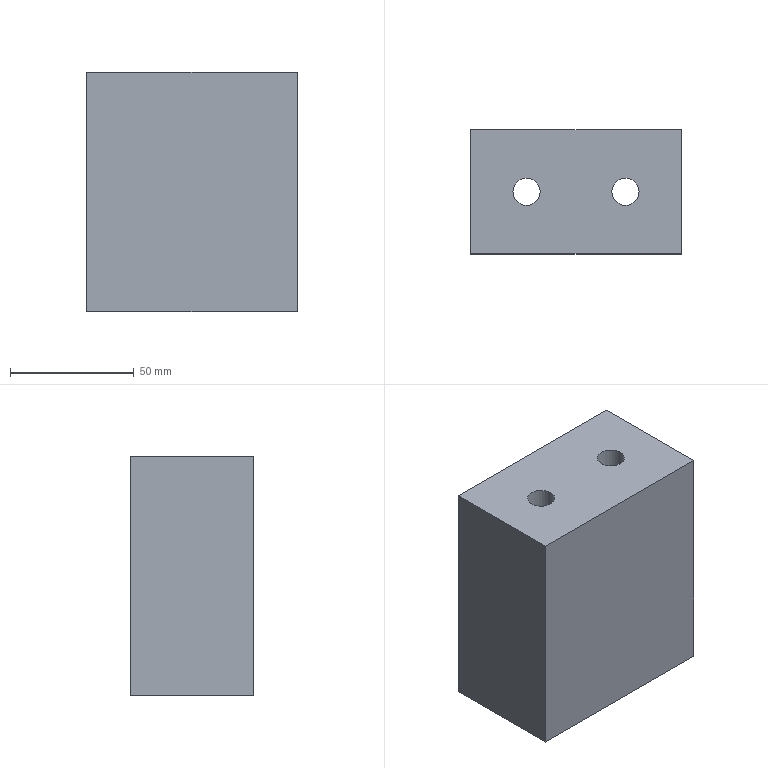Part | STEP file | PN_0040_id1406_x_t | 1 solid | 12 faces | box 85 x 50 x 97 mm | volume 372174 mm3 | plane 8 | cylinder 4 | commonest cylinder face diameters 11 x2 17 x2
STEP:
#1=CARTESIAN_POINT('',(-370.,-242.5,105.));
#2=VERTEX_POINT('',#1);
#3=CARTESIAN_POINT('',(-285.,-242.5,105.));
#4=VERTEX_POINT('',#3);
#5=CARTESIAN_POINT('',(-327.5,-242.5,105.));
#6=DIRECTION('',(1.,0.,0.));
#7=VECTOR('',#6,1.);
#8=LINE('',#5,#7);
#9=EDGE_CURVE('',#2,#4,#8,.T.);
#10=ORIENTED_EDGE('',*,*,#9,.T.);
#11=CARTESIAN_POINT('',(-285.,-242.5,8.));
#12=VERTEX_POINT('',#11);
#13=CARTESIAN_POINT('',(-285.,-242.5,6.));
#14=DIRECTION('',(0.,0.,-1.));
#15=VECTOR('',#14,1.);
#16=LINE('',#13,#15);
#17=EDGE_CURVE('',#4,#12,#16,.T.);
#18=ORIENTED_EDGE('',*,*,#17,.T.);
#19=CARTESIAN_POINT('',(-370.,-242.5,8.));
#20=VERTEX_POINT('',#19);
#21=CARTESIAN_POINT('',(-327.5,-242.5,8.));
#22=DIRECTION('',(-1.,0.,0.));
#23=VECTOR('',#22,1.);
#24=LINE('',#21,#23);
#25=EDGE_CURVE('',#12,#20,#24,.T.);
#26=ORIENTED_EDGE('',*,*,#25,.T.);
#27=CARTESIAN_POINT('',(-370.,-242.5,6.));
#28=DIRECTION('',(0.,0.,-1.));
#29=VECTOR('',#28,1.);
#30=LINE('',#27,#29);
#31=EDGE_CURVE('',#2,#20,#30,.T.);
#32=ORIENTED_EDGE('',*,*,#31,.F.);
#33=EDGE_LOOP('',(#10,#18,#26,#32));
#34=FACE_OUTER_BOUND('',#33,.T.);
#35=CARTESIAN_POINT('',(-327.5,-242.5,6.));
#36=DIRECTION('',(0.,1.,0.));
#37=DIRECTION('',(0.,0.,1.));
#38=AXIS2_PLACEMENT_3D('',#35,#36,#37);
#39=PLANE('',#38);
#40=ADVANCED_FACE('',(#34),#39,.T.);
#41=CARTESIAN_POINT('',(-370.,-292.5,105.));
#42=VERTEX_POINT('',#41);
#43=CARTESIAN_POINT('',(-370.,-267.5,105.));
#44=DIRECTION('',(0.,1.,0.));
#45=VECTOR('',#44,1.);
#46=LINE('',#43,#45);
#47=EDGE_CURVE('',#42,#2,#46,.T.);
#48=ORIENTED_EDGE('',*,*,#47,.T.);
#49=ORIENTED_EDGE('',*,*,#31,.T.);
#50=CARTESIAN_POINT('',(-370.,-292.5,8.));
#51=VERTEX_POINT('',#50);
#52=CARTESIAN_POINT('',(-370.,-267.5,8.));
#53=DIRECTION('',(0.,-1.,0.));
#54=VECTOR('',#53,1.);
#55=LINE('',#52,#54);
#56=EDGE_CURVE('',#20,#51,#55,.T.);
#57=ORIENTED_EDGE('',*,*,#56,.T.);
#58=CARTESIAN_POINT('',(-370.,-292.5,6.));
#59=DIRECTION('',(0.,0.,-1.));
#60=VECTOR('',#59,1.);
#61=LINE('',#58,#60);
#62=EDGE_CURVE('',#42,#51,#61,.T.);
#63=ORIENTED_EDGE('',*,*,#62,.F.);
#64=EDGE_LOOP('',(#48,#49,#57,#63));
#65=FACE_OUTER_BOUND('',#64,.T.);
#66=CARTESIAN_POINT('',(-370.,-267.5,6.));
#67=DIRECTION('',(-1.,0.,0.));
#68=DIRECTION('',(0.,0.,1.));
#69=AXIS2_PLACEMENT_3D('',#66,#67,#68);
#70=PLANE('',#69);
#71=ADVANCED_FACE('',(#65),#70,.T.);
#72=CARTESIAN_POINT('',(-285.,-292.5,8.));
#73=VERTEX_POINT('',#72);
#74=CARTESIAN_POINT('',(-327.5,-292.5,8.));
#75=DIRECTION('',(1.,0.,0.));
#76=VECTOR('',#75,1.);
#77=LINE('',#74,#76);
#78=EDGE_CURVE('',#51,#73,#77,.T.);
#79=ORIENTED_EDGE('',*,*,#78,.T.);
#80=CARTESIAN_POINT('',(-285.,-292.5,105.));
#81=VERTEX_POINT('',#80);
#82=CARTESIAN_POINT('',(-285.,-292.5,6.));
#83=DIRECTION('',(0.,0.,-1.));
#84=VECTOR('',#83,1.);
#85=LINE('',#82,#84);
#86=EDGE_CURVE('',#81,#73,#85,.T.);
#87=ORIENTED_EDGE('',*,*,#86,.F.);
#88=CARTESIAN_POINT('',(-327.5,-292.5,105.));
#89=DIRECTION('',(-1.,0.,0.));
#90=VECTOR('',#89,1.);
#91=LINE('',#88,#90);
#92=EDGE_CURVE('',#81,#42,#91,.T.);
#93=ORIENTED_EDGE('',*,*,#92,.T.);
#94=ORIENTED_EDGE('',*,*,#62,.T.);
#95=EDGE_LOOP('',(#79,#87,#93,#94));
#96=FACE_OUTER_BOUND('',#95,.T.);
#97=CARTESIAN_POINT('',(-327.5,-292.5,6.));
#98=DIRECTION('',(0.,-1.,0.));
#99=DIRECTION('',(0.,0.,-1.));
#100=AXIS2_PLACEMENT_3D('',#97,#98,#99);
#101=PLANE('',#100);
#102=ADVANCED_FACE('',(#96),#101,.T.);
#103=CARTESIAN_POINT('',(-285.,-267.5,8.));
#104=DIRECTION('',(0.,1.,0.));
#105=VECTOR('',#104,1.);
#106=LINE('',#103,#105);
#107=EDGE_CURVE('',#73,#12,#106,.T.);
#108=ORIENTED_EDGE('',*,*,#107,.T.);
#109=ORIENTED_EDGE('',*,*,#17,.F.);
#110=CARTESIAN_POINT('',(-285.,-267.5,105.));
#111=DIRECTION('',(0.,-1.,0.));
#112=VECTOR('',#111,1.);
#113=LINE('',#110,#112);
#114=EDGE_CURVE('',#4,#81,#113,.T.);
#115=ORIENTED_EDGE('',*,*,#114,.T.);
#116=ORIENTED_EDGE('',*,*,#86,.T.);
#117=EDGE_LOOP('',(#108,#109,#115,#116));
#118=FACE_OUTER_BOUND('',#117,.T.);
#119=CARTESIAN_POINT('',(-285.,-267.5,6.));
#120=DIRECTION('',(1.,0.,0.));
#121=DIRECTION('',(0.,0.,-1.));
#122=AXIS2_PLACEMENT_3D('',#119,#120,#121);
#123=PLANE('',#122);
#124=ADVANCED_FACE('',(#118),#123,.T.);
#125=CARTESIAN_POINT('',(-356.,-267.5,8.));
#126=VERTEX_POINT('',#125);
#127=CARTESIAN_POINT('',(-347.5,-267.5,8.));
#128=DIRECTION('',(0.,0.,-1.));
#129=DIRECTION('',(-1.,0.,0.));
#130=AXIS2_PLACEMENT_3D('',#127,#128,#129);
#131=CIRCLE('',#130,8.5);
#132=EDGE_CURVE('',#126,#126,#131,.T.);
#133=ORIENTED_EDGE('',*,*,#132,.F.);
#134=EDGE_LOOP('',(#133));
#135=FACE_BOUND('',#134,.T.);
#136=CARTESIAN_POINT('',(-316.,-267.5,8.));
#137=VERTEX_POINT('',#136);
#138=CARTESIAN_POINT('',(-307.5,-267.5,8.));
#139=DIRECTION('',(0.,0.,-1.));
#140=DIRECTION('',(-1.,0.,0.));
#141=AXIS2_PLACEMENT_3D('',#138,#139,#140);
#142=CIRCLE('',#141,8.5);
#143=EDGE_CURVE('',#137,#137,#142,.T.);
#144=ORIENTED_EDGE('',*,*,#143,.F.);
#145=EDGE_LOOP('',(#144));
#146=FACE_BOUND('',#145,.T.);
#147=ORIENTED_EDGE('',*,*,#25,.F.);
#148=ORIENTED_EDGE('',*,*,#107,.F.);
#149=ORIENTED_EDGE('',*,*,#78,.F.);
#150=ORIENTED_EDGE('',*,*,#56,.F.);
#151=EDGE_LOOP('',(#147,#148,#149,#150));
#152=FACE_BOUND('',#151,.T.);
#153=CARTESIAN_POINT('',(-327.5,-267.5,8.));
#154=DIRECTION('',(0.,0.,-1.));
#155=DIRECTION('',(-1.,0.,0.));
#156=AXIS2_PLACEMENT_3D('',#153,#154,#155);
#157=PLANE('',#156);
#158=ADVANCED_FACE('',(#135,#146,#152),#157,.T.);
#159=CARTESIAN_POINT('',(-342.,-267.5,105.));
#160=VERTEX_POINT('',#159);
#161=CARTESIAN_POINT('',(-347.5,-267.5,105.));
#162=DIRECTION('',(0.,0.,1.));
#163=DIRECTION('',(1.,0.,0.));
#164=AXIS2_PLACEMENT_3D('',#161,#162,#163);
#165=CIRCLE('',#164,5.5);
#166=EDGE_CURVE('',#160,#160,#165,.T.);
#167=ORIENTED_EDGE('',*,*,#166,.F.);
#168=EDGE_LOOP('',(#167));
#169=FACE_BOUND('',#168,.T.);
#170=CARTESIAN_POINT('',(-302.,-267.5,105.));
#171=VERTEX_POINT('',#170);
#172=CARTESIAN_POINT('',(-307.5,-267.5,105.));
#173=DIRECTION('',(0.,0.,1.));
#174=DIRECTION('',(1.,0.,0.));
#175=AXIS2_PLACEMENT_3D('',#172,#173,#174);
#176=CIRCLE('',#175,5.5);
#177=EDGE_CURVE('',#171,#171,#176,.T.);
#178=ORIENTED_EDGE('',*,*,#177,.F.);
#179=EDGE_LOOP('',(#178));
#180=FACE_BOUND('',#179,.T.);
#181=ORIENTED_EDGE('',*,*,#114,.F.);
#182=ORIENTED_EDGE('',*,*,#9,.F.);
#183=ORIENTED_EDGE('',*,*,#47,.F.);
#184=ORIENTED_EDGE('',*,*,#92,.F.);
#185=EDGE_LOOP('',(#181,#182,#183,#184));
#186=FACE_BOUND('',#185,.T.);
#187=CARTESIAN_POINT('',(454.3,202.5,105.));
#188=DIRECTION('',(0.,0.,1.));
#189=DIRECTION('',(1.,0.,0.));
#190=AXIS2_PLACEMENT_3D('',#187,#188,#189);
#191=PLANE('',#190);
#192=ADVANCED_FACE('',(#169,#180,#186),#191,.T.);
#193=CARTESIAN_POINT('',(-313.,-267.5,90.));
#194=VERTEX_POINT('',#193);
#195=CARTESIAN_POINT('',(-307.5,-267.5,90.));
#196=DIRECTION('',(0.,0.,-1.));
#197=DIRECTION('',(-1.,0.,0.));
#198=AXIS2_PLACEMENT_3D('',#195,#196,#197);
#199=CIRCLE('',#198,5.5);
#200=EDGE_CURVE('',#194,#194,#199,.T.);
#201=ORIENTED_EDGE('',*,*,#200,.T.);
#202=EDGE_LOOP('',(#201));
#203=FACE_BOUND('',#202,.T.);
#204=ORIENTED_EDGE('',*,*,#177,.T.);
#205=EDGE_LOOP('',(#204));
#206=FACE_BOUND('',#205,.T.);
#207=CARTESIAN_POINT('',(-307.5,-267.5,105.));
#208=DIRECTION('',(0.,0.,-1.));
#209=DIRECTION('',(1.,0.,0.));
#210=AXIS2_PLACEMENT_3D('',#207,#208,#209);
#211=CYLINDRICAL_SURFACE('',#210,5.5);
#212=ADVANCED_FACE('',(#203,#206),#211,.F.);
#213=ORIENTED_EDGE('',*,*,#200,.F.);
#214=EDGE_LOOP('',(#213));
#215=FACE_BOUND('',#214,.T.);
#216=CARTESIAN_POINT('',(-299.,-267.5,90.));
#217=VERTEX_POINT('',#216);
#218=CARTESIAN_POINT('',(-307.5,-267.5,90.));
#219=DIRECTION('',(0.,0.,-1.));
#220=DIRECTION('',(1.,0.,0.));
#221=AXIS2_PLACEMENT_3D('',#218,#219,#220);
#222=CIRCLE('',#221,8.5);
#223=EDGE_CURVE('',#217,#217,#222,.T.);
#224=ORIENTED_EDGE('',*,*,#223,.T.);
#225=EDGE_LOOP('',(#224));
#226=FACE_BOUND('',#225,.T.);
#227=CARTESIAN_POINT('',(-307.5,-267.5,90.));
#228=DIRECTION('',(0.,0.,1.));
#229=DIRECTION('',(-1.,0.,0.));
#230=AXIS2_PLACEMENT_3D('',#227,#228,#229);
#231=PLANE('',#230);
#232=ADVANCED_FACE('',(#215,#226),#231,.F.);
#233=ORIENTED_EDGE('',*,*,#143,.T.);
#234=EDGE_LOOP('',(#233));
#235=FACE_BOUND('',#234,.T.);
#236=ORIENTED_EDGE('',*,*,#223,.F.);
#237=EDGE_LOOP('',(#236));
#238=FACE_BOUND('',#237,.T.);
#239=CARTESIAN_POINT('',(-307.5,-267.5,90.));
#240=DIRECTION('',(0.,0.,-1.));
#241=DIRECTION('',(1.,0.,0.));
#242=AXIS2_PLACEMENT_3D('',#239,#240,#241);
#243=CYLINDRICAL_SURFACE('',#242,8.5);
#244=ADVANCED_FACE('',(#235,#238),#243,.F.);
#245=CARTESIAN_POINT('',(-353.,-267.5,90.));
#246=VERTEX_POINT('',#245);
#247=CARTESIAN_POINT('',(-347.5,-267.5,90.));
#248=DIRECTION('',(0.,0.,-1.));
#249=DIRECTION('',(-1.,0.,0.));
#250=AXIS2_PLACEMENT_3D('',#247,#248,#249);
#251=CIRCLE('',#250,5.5);
#252=EDGE_CURVE('',#246,#246,#251,.T.);
#253=ORIENTED_EDGE('',*,*,#252,.T.);
#254=EDGE_LOOP('',(#253));
#255=FACE_BOUND('',#254,.T.);
#256=ORIENTED_EDGE('',*,*,#166,.T.);
#257=EDGE_LOOP('',(#256));
#258=FACE_BOUND('',#257,.T.);
#259=CARTESIAN_POINT('',(-347.5,-267.5,105.));
#260=DIRECTION('',(0.,0.,-1.));
#261=DIRECTION('',(1.,0.,0.));
#262=AXIS2_PLACEMENT_3D('',#259,#260,#261);
#263=CYLINDRICAL_SURFACE('',#262,5.5);
#264=ADVANCED_FACE('',(#255,#258),#263,.F.);
#265=ORIENTED_EDGE('',*,*,#252,.F.);
#266=EDGE_LOOP('',(#265));
#267=FACE_BOUND('',#266,.T.);
#268=CARTESIAN_POINT('',(-339.,-267.5,90.));
#269=VERTEX_POINT('',#268);
#270=CARTESIAN_POINT('',(-347.5,-267.5,90.));
#271=DIRECTION('',(0.,0.,-1.));
#272=DIRECTION('',(1.,0.,0.));
#273=AXIS2_PLACEMENT_3D('',#270,#271,#272);
#274=CIRCLE('',#273,8.5);
#275=EDGE_CURVE('',#269,#269,#274,.T.);
#276=ORIENTED_EDGE('',*,*,#275,.T.);
#277=EDGE_LOOP('',(#276));
#278=FACE_BOUND('',#277,.T.);
#279=CARTESIAN_POINT('',(-347.5,-267.5,90.));
#280=DIRECTION('',(0.,0.,1.));
#281=DIRECTION('',(-1.,0.,0.));
#282=AXIS2_PLACEMENT_3D('',#279,#280,#281);
#283=PLANE('',#282);
#284=ADVANCED_FACE('',(#267,#278),#283,.F.);
#285=ORIENTED_EDGE('',*,*,#132,.T.);
#286=EDGE_LOOP('',(#285));
#287=FACE_BOUND('',#286,.T.);
#288=ORIENTED_EDGE('',*,*,#275,.F.);
#289=EDGE_LOOP('',(#288));
#290=FACE_BOUND('',#289,.T.);
#291=CARTESIAN_POINT('',(-347.5,-267.5,90.));
#292=DIRECTION('',(0.,0.,-1.));
#293=DIRECTION('',(1.,0.,0.));
#294=AXIS2_PLACEMENT_3D('',#291,#292,#293);
#295=CYLINDRICAL_SURFACE('',#294,8.5);
#296=ADVANCED_FACE('',(#287,#290),#295,.F.);
#297=CLOSED_SHELL('',(#40,#71,#102,#124,#158,#192,#212,#232,#244,#264,#284,#296));
#298=MANIFOLD_SOLID_BREP('',#297);
#299=(LENGTH_UNIT()NAMED_UNIT(*)SI_UNIT(.MILLI.,.METRE.));
#300=UNCERTAINTY_MEASURE_WITH_UNIT(LENGTH_MEASURE(0.00002),#299,'','');
#301=(NAMED_UNIT(*)PLANE_ANGLE_UNIT()SI_UNIT($,.RADIAN.));
#302=PLANE_ANGLE_MEASURE_WITH_UNIT(PLANE_ANGLE_MEASURE(0.01745),#301);
#303=DIMENSIONAL_EXPONENTS(0.,0.,0.,0.,0.,0.,0.);
#304=(CONVERSION_BASED_UNIT('DEGREE',#302)NAMED_UNIT(#303)PLANE_ANGLE_UNIT());
#305=(NAMED_UNIT(*)SI_UNIT($,.STERADIAN.)SOLID_ANGLE_UNIT());
#306=(GEOMETRIC_REPRESENTATION_CONTEXT(3)GLOBAL_UNCERTAINTY_ASSIGNED_CONTEXT((#300))GLOBAL_UNIT_ASSIGNED_CONTEXT((#299,#304,#305))REPRESENTATION_CONTEXT('',''));
#307=ADVANCED_BREP_SHAPE_REPRESENTATION('',(#298),#306);